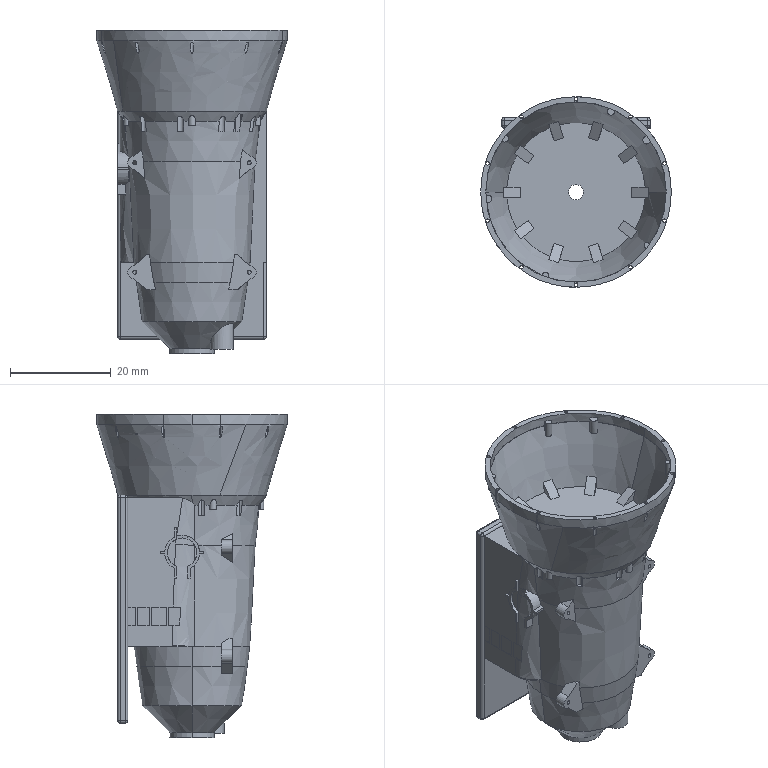Part | SolidWorks | features ICE 18, Blend 7, DelFace 4, Fillet 4, CirPattern 2, MirrorPattern 2, BlendCut 1, Extrusion 1, Rib 1, Shell 1 | 1 solid | 334 faces | box 37.751 x 37.751 x 64.09 mm | volume 13251 mm3 | plane 174 | cylinder 108 | cone 30 | sphere 8 | torus 7 | spline 7 | commonest cylinder face diameters 0.696 x20 1.299 x18 1 x15 0.768 x8 1.38 x8 6.936 x5